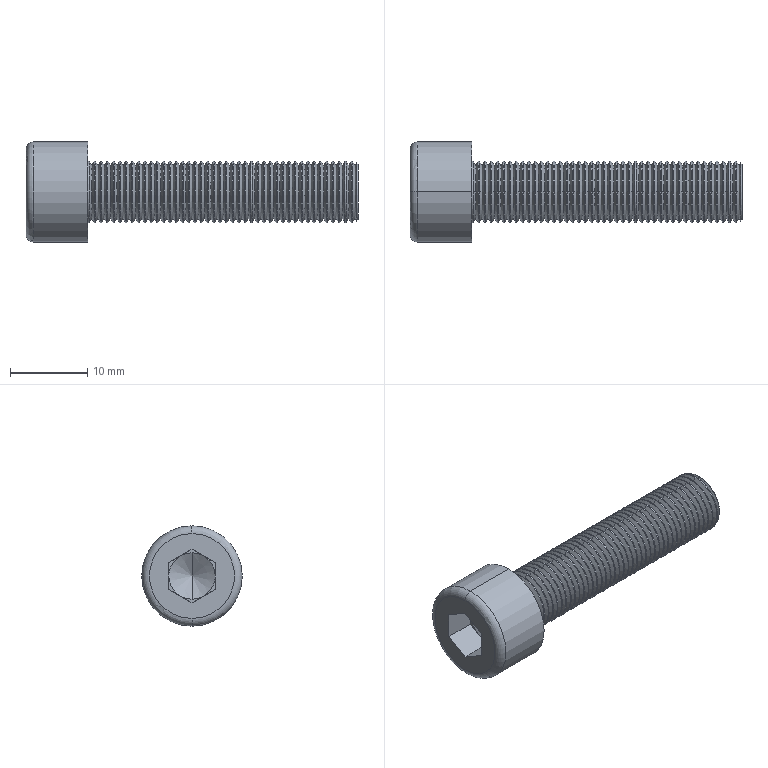Part | STEP file | PN_0040_Default<As Machined> | 1 solid | 281 faces | box 43 x 13 x 13 mm | volume 2467 mm3 | cone 176 | cylinder 88 | plane 15 | torus 2 | commonest cylinder face diameters 8 x86 13 x2